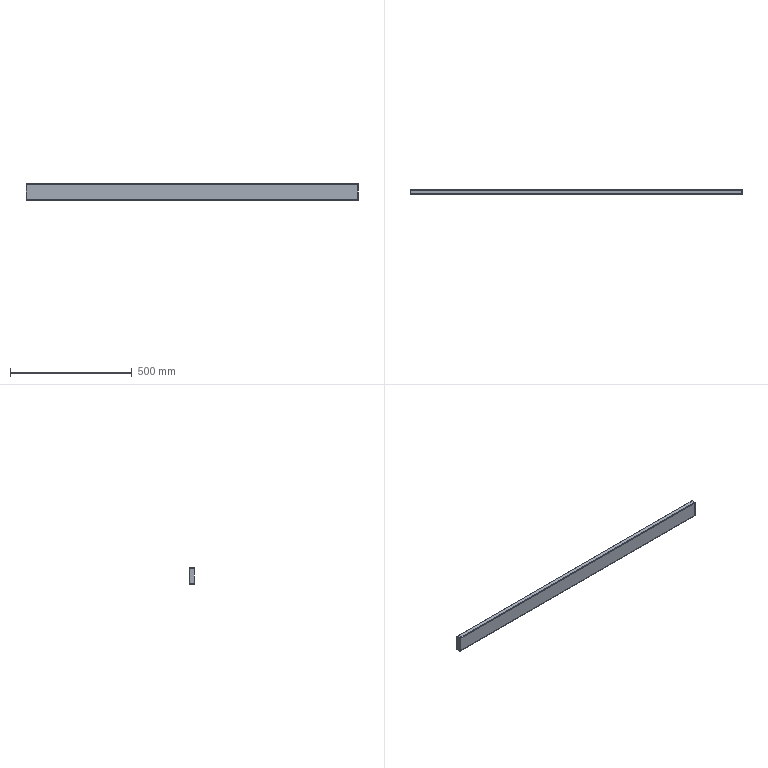Part | SolidWorks | features FlatPattern 5, EdgeFlange 2, SMBaseFlange 2, SheetMetal 2, HoleWzd 1, ICE 1, LPattern 1, MirrorSolid 1 | 7 solids | 90 faces | box 1364 x 20 x 68 mm | volume 272677 mm3 | plane 66 | cylinder 24 | commonest cylinder face diameters 7 x12 5 x8 4 x4